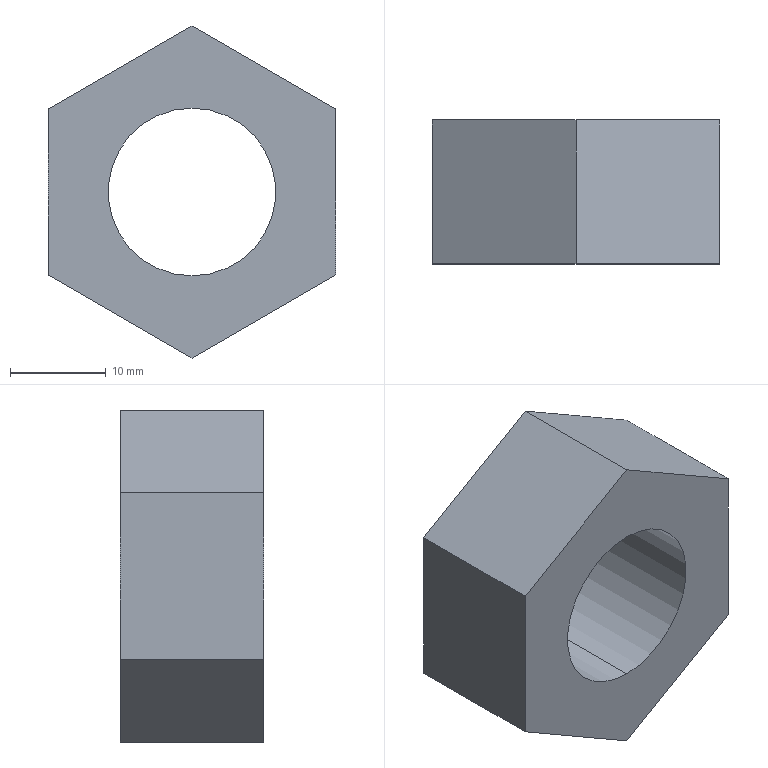Part | SolidWorks | features Extrusion 1, HoleWzd 1 | 1 solid | 10 faces | box 30 x 15 x 34.641 mm | volume 8083 mm3 | plane 8 | cylinder 2 | commonest cylinder face diameters 17.5 x2
STEP:
#1=CARTESIAN_POINT('',(0.,0.,-8.75));
#2=VERTEX_POINT('',#1);
#3=CARTESIAN_POINT('',(0.,0.,8.75));
#4=VERTEX_POINT('',#3);
#5=CARTESIAN_POINT('',(0.,0.,0.));
#6=DIRECTION('',(0.,1.,0.));
#7=DIRECTION('',(0.,0.,1.));
#8=AXIS2_PLACEMENT_3D('',#5,#6,#7);
#9=CIRCLE('',#8,8.75);
#10=EDGE_CURVE('',#2,#4,#9,.T.);
#11=ORIENTED_EDGE('',*,*,#10,.F.);
#12=CARTESIAN_POINT('',(0.,15.,-8.75));
#13=VERTEX_POINT('',#12);
#14=CARTESIAN_POINT('',(0.,15.,-8.75));
#15=DIRECTION('',(0.,1.,0.));
#16=VECTOR('',#15,1000.);
#17=LINE('',#14,#16);
#18=EDGE_CURVE('',#2,#13,#17,.T.);
#19=ORIENTED_EDGE('',*,*,#18,.T.);
#20=CARTESIAN_POINT('',(0.,15.,8.75));
#21=VERTEX_POINT('',#20);
#22=CARTESIAN_POINT('',(0.,15.,0.));
#23=DIRECTION('',(0.,1.,0.));
#24=DIRECTION('',(0.,0.,1.));
#25=AXIS2_PLACEMENT_3D('',#22,#23,#24);
#26=CIRCLE('',#25,8.75);
#27=EDGE_CURVE('',#13,#21,#26,.T.);
#28=ORIENTED_EDGE('',*,*,#27,.T.);
#29=CARTESIAN_POINT('',(0.,15.,8.75));
#30=DIRECTION('',(0.,1.,0.));
#31=VECTOR('',#30,1000.);
#32=LINE('',#29,#31);
#33=EDGE_CURVE('',#4,#21,#32,.T.);
#34=ORIENTED_EDGE('',*,*,#33,.F.);
#35=EDGE_LOOP('',(#11,#19,#28,#34));
#36=FACE_OUTER_BOUND('',#35,.T.);
#37=CARTESIAN_POINT('',(0.,15.,0.));
#38=DIRECTION('',(0.,1.,0.));
#39=DIRECTION('',(0.,0.,1.));
#40=AXIS2_PLACEMENT_3D('',#37,#38,#39);
#41=CYLINDRICAL_SURFACE('',#40,8.75);
#42=ADVANCED_FACE('',(#36),#41,.F.);
#43=CARTESIAN_POINT('',(15.,0.,-8.66));
#44=VERTEX_POINT('',#43);
#45=CARTESIAN_POINT('',(0.,0.,-17.321));
#46=VERTEX_POINT('',#45);
#47=CARTESIAN_POINT('',(15.,0.,-8.66));
#48=DIRECTION('',(-0.866,0.,-0.5));
#49=VECTOR('',#48,1000.);
#50=LINE('',#47,#49);
#51=EDGE_CURVE('',#44,#46,#50,.T.);
#52=ORIENTED_EDGE('',*,*,#51,.T.);
#53=CARTESIAN_POINT('',(0.,15.,-17.321));
#54=VERTEX_POINT('',#53);
#55=CARTESIAN_POINT('',(0.,15.,-17.321));
#56=DIRECTION('',(0.,-1.,0.));
#57=VECTOR('',#56,1000.);
#58=LINE('',#55,#57);
#59=EDGE_CURVE('',#54,#46,#58,.T.);
#60=ORIENTED_EDGE('',*,*,#59,.F.);
#61=CARTESIAN_POINT('',(15.,15.,-8.66));
#62=VERTEX_POINT('',#61);
#63=CARTESIAN_POINT('',(15.,15.,-8.66));
#64=DIRECTION('',(-0.866,0.,-0.5));
#65=VECTOR('',#64,1000.);
#66=LINE('',#63,#65);
#67=EDGE_CURVE('',#62,#54,#66,.T.);
#68=ORIENTED_EDGE('',*,*,#67,.F.);
#69=CARTESIAN_POINT('',(15.,15.,-8.66));
#70=DIRECTION('',(0.,-1.,0.));
#71=VECTOR('',#70,1000.);
#72=LINE('',#69,#71);
#73=EDGE_CURVE('',#62,#44,#72,.T.);
#74=ORIENTED_EDGE('',*,*,#73,.T.);
#75=EDGE_LOOP('',(#52,#60,#68,#74));
#76=FACE_OUTER_BOUND('',#75,.T.);
#77=CARTESIAN_POINT('',(15.,15.,-8.66));
#78=DIRECTION('',(-0.5,0.,0.866));
#79=DIRECTION('',(0.866,0.,0.5));
#80=AXIS2_PLACEMENT_3D('',#77,#78,#79);
#81=PLANE('',#80);
#82=ADVANCED_FACE('',(#76),#81,.F.);
#83=CARTESIAN_POINT('',(-15.,0.,-8.66));
#84=VERTEX_POINT('',#83);
#85=CARTESIAN_POINT('',(0.,0.,-17.321));
#86=DIRECTION('',(-0.866,0.,0.5));
#87=VECTOR('',#86,1000.);
#88=LINE('',#85,#87);
#89=EDGE_CURVE('',#46,#84,#88,.T.);
#90=ORIENTED_EDGE('',*,*,#89,.T.);
#91=CARTESIAN_POINT('',(-15.,15.,-8.66));
#92=VERTEX_POINT('',#91);
#93=CARTESIAN_POINT('',(-15.,15.,-8.66));
#94=DIRECTION('',(0.,-1.,0.));
#95=VECTOR('',#94,1000.);
#96=LINE('',#93,#95);
#97=EDGE_CURVE('',#92,#84,#96,.T.);
#98=ORIENTED_EDGE('',*,*,#97,.F.);
#99=CARTESIAN_POINT('',(0.,15.,-17.321));
#100=DIRECTION('',(-0.866,0.,0.5));
#101=VECTOR('',#100,1000.);
#102=LINE('',#99,#101);
#103=EDGE_CURVE('',#54,#92,#102,.T.);
#104=ORIENTED_EDGE('',*,*,#103,.F.);
#105=ORIENTED_EDGE('',*,*,#59,.T.);
#106=EDGE_LOOP('',(#90,#98,#104,#105));
#107=FACE_OUTER_BOUND('',#106,.T.);
#108=CARTESIAN_POINT('',(0.,15.,-17.321));
#109=DIRECTION('',(0.5,0.,0.866));
#110=DIRECTION('',(0.866,0.,-0.5));
#111=AXIS2_PLACEMENT_3D('',#108,#109,#110);
#112=PLANE('',#111);
#113=ADVANCED_FACE('',(#107),#112,.F.);
#114=CARTESIAN_POINT('',(-15.,0.,8.66));
#115=VERTEX_POINT('',#114);
#116=CARTESIAN_POINT('',(-15.,0.,-8.66));
#117=DIRECTION('',(0.,0.,1.));
#118=VECTOR('',#117,1000.);
#119=LINE('',#116,#118);
#120=EDGE_CURVE('',#84,#115,#119,.T.);
#121=ORIENTED_EDGE('',*,*,#120,.T.);
#122=CARTESIAN_POINT('',(-15.,15.,8.66));
#123=VERTEX_POINT('',#122);
#124=CARTESIAN_POINT('',(-15.,15.,8.66));
#125=DIRECTION('',(0.,-1.,0.));
#126=VECTOR('',#125,1000.);
#127=LINE('',#124,#126);
#128=EDGE_CURVE('',#123,#115,#127,.T.);
#129=ORIENTED_EDGE('',*,*,#128,.F.);
#130=CARTESIAN_POINT('',(-15.,15.,-8.66));
#131=DIRECTION('',(0.,0.,1.));
#132=VECTOR('',#131,1000.);
#133=LINE('',#130,#132);
#134=EDGE_CURVE('',#92,#123,#133,.T.);
#135=ORIENTED_EDGE('',*,*,#134,.F.);
#136=ORIENTED_EDGE('',*,*,#97,.T.);
#137=EDGE_LOOP('',(#121,#129,#135,#136));
#138=FACE_OUTER_BOUND('',#137,.T.);
#139=CARTESIAN_POINT('',(-15.,15.,-8.66));
#140=DIRECTION('',(1.,0.,0.));
#141=DIRECTION('',(0.,0.,-1.));
#142=AXIS2_PLACEMENT_3D('',#139,#140,#141);
#143=PLANE('',#142);
#144=ADVANCED_FACE('',(#138),#143,.F.);
#145=CARTESIAN_POINT('',(0.,0.,17.321));
#146=VERTEX_POINT('',#145);
#147=CARTESIAN_POINT('',(-15.,0.,8.66));
#148=DIRECTION('',(0.866,0.,0.5));
#149=VECTOR('',#148,1000.);
#150=LINE('',#147,#149);
#151=EDGE_CURVE('',#115,#146,#150,.T.);
#152=ORIENTED_EDGE('',*,*,#151,.T.);
#153=CARTESIAN_POINT('',(0.,15.,17.321));
#154=VERTEX_POINT('',#153);
#155=CARTESIAN_POINT('',(0.,15.,17.321));
#156=DIRECTION('',(0.,-1.,0.));
#157=VECTOR('',#156,1000.);
#158=LINE('',#155,#157);
#159=EDGE_CURVE('',#154,#146,#158,.T.);
#160=ORIENTED_EDGE('',*,*,#159,.F.);
#161=CARTESIAN_POINT('',(-15.,15.,8.66));
#162=DIRECTION('',(0.866,0.,0.5));
#163=VECTOR('',#162,1000.);
#164=LINE('',#161,#163);
#165=EDGE_CURVE('',#123,#154,#164,.T.);
#166=ORIENTED_EDGE('',*,*,#165,.F.);
#167=ORIENTED_EDGE('',*,*,#128,.T.);
#168=EDGE_LOOP('',(#152,#160,#166,#167));
#169=FACE_OUTER_BOUND('',#168,.T.);
#170=CARTESIAN_POINT('',(-15.,15.,8.66));
#171=DIRECTION('',(0.5,0.,-0.866));
#172=DIRECTION('',(-0.866,0.,-0.5));
#173=AXIS2_PLACEMENT_3D('',#170,#171,#172);
#174=PLANE('',#173);
#175=ADVANCED_FACE('',(#169),#174,.F.);
#176=CARTESIAN_POINT('',(15.,0.,8.66));
#177=VERTEX_POINT('',#176);
#178=CARTESIAN_POINT('',(0.,0.,17.321));
#179=DIRECTION('',(0.866,0.,-0.5));
#180=VECTOR('',#179,1000.);
#181=LINE('',#178,#180);
#182=EDGE_CURVE('',#146,#177,#181,.T.);
#183=ORIENTED_EDGE('',*,*,#182,.T.);
#184=CARTESIAN_POINT('',(15.,15.,8.66));
#185=VERTEX_POINT('',#184);
#186=CARTESIAN_POINT('',(15.,15.,8.66));
#187=DIRECTION('',(0.,-1.,0.));
#188=VECTOR('',#187,1000.);
#189=LINE('',#186,#188);
#190=EDGE_CURVE('',#185,#177,#189,.T.);
#191=ORIENTED_EDGE('',*,*,#190,.F.);
#192=CARTESIAN_POINT('',(0.,15.,17.321));
#193=DIRECTION('',(0.866,0.,-0.5));
#194=VECTOR('',#193,1000.);
#195=LINE('',#192,#194);
#196=EDGE_CURVE('',#154,#185,#195,.T.);
#197=ORIENTED_EDGE('',*,*,#196,.F.);
#198=ORIENTED_EDGE('',*,*,#159,.T.);
#199=EDGE_LOOP('',(#183,#191,#197,#198));
#200=FACE_OUTER_BOUND('',#199,.T.);
#201=CARTESIAN_POINT('',(0.,15.,17.321));
#202=DIRECTION('',(-0.5,0.,-0.866));
#203=DIRECTION('',(-0.866,0.,0.5));
#204=AXIS2_PLACEMENT_3D('',#201,#202,#203);
#205=PLANE('',#204);
#206=ADVANCED_FACE('',(#200),#205,.F.);
#207=CARTESIAN_POINT('',(15.,0.,8.66));
#208=DIRECTION('',(0.,0.,-1.));
#209=VECTOR('',#208,1000.);
#210=LINE('',#207,#209);
#211=EDGE_CURVE('',#177,#44,#210,.T.);
#212=ORIENTED_EDGE('',*,*,#211,.T.);
#213=ORIENTED_EDGE('',*,*,#73,.F.);
#214=CARTESIAN_POINT('',(15.,15.,8.66));
#215=DIRECTION('',(0.,0.,-1.));
#216=VECTOR('',#215,1000.);
#217=LINE('',#214,#216);
#218=EDGE_CURVE('',#185,#62,#217,.T.);
#219=ORIENTED_EDGE('',*,*,#218,.F.);
#220=ORIENTED_EDGE('',*,*,#190,.T.);
#221=EDGE_LOOP('',(#212,#213,#219,#220));
#222=FACE_OUTER_BOUND('',#221,.T.);
#223=CARTESIAN_POINT('',(15.,15.,8.66));
#224=DIRECTION('',(-1.,0.,0.));
#225=DIRECTION('',(0.,0.,1.));
#226=AXIS2_PLACEMENT_3D('',#223,#224,#225);
#227=PLANE('',#226);
#228=ADVANCED_FACE('',(#222),#227,.F.);
#229=CARTESIAN_POINT('',(0.,15.,0.));
#230=DIRECTION('',(0.,1.,0.));
#231=DIRECTION('',(0.,0.,1.));
#232=AXIS2_PLACEMENT_3D('',#229,#230,#231);
#233=CIRCLE('',#232,8.75);
#234=EDGE_CURVE('',#21,#13,#233,.T.);
#235=ORIENTED_EDGE('',*,*,#234,.F.);
#236=ORIENTED_EDGE('',*,*,#27,.F.);
#237=EDGE_LOOP('',(#235,#236));
#238=FACE_BOUND('',#237,.T.);
#239=ORIENTED_EDGE('',*,*,#67,.T.);
#240=ORIENTED_EDGE('',*,*,#103,.T.);
#241=ORIENTED_EDGE('',*,*,#134,.T.);
#242=ORIENTED_EDGE('',*,*,#165,.T.);
#243=ORIENTED_EDGE('',*,*,#196,.T.);
#244=ORIENTED_EDGE('',*,*,#218,.T.);
#245=EDGE_LOOP('',(#239,#240,#241,#242,#243,#244));
#246=FACE_OUTER_BOUND('',#245,.T.);
#247=CARTESIAN_POINT('',(0.,15.,0.));
#248=DIRECTION('',(0.,1.,0.));
#249=DIRECTION('',(0.,0.,1.));
#250=AXIS2_PLACEMENT_3D('',#247,#248,#249);
#251=PLANE('',#250);
#252=ADVANCED_FACE('',(#238,#246),#251,.T.);
#253=CARTESIAN_POINT('',(0.,0.,0.));
#254=DIRECTION('',(0.,1.,0.));
#255=DIRECTION('',(0.,0.,1.));
#256=AXIS2_PLACEMENT_3D('',#253,#254,#255);
#257=CIRCLE('',#256,8.75);
#258=EDGE_CURVE('',#4,#2,#257,.T.);
#259=ORIENTED_EDGE('',*,*,#258,.T.);
#260=ORIENTED_EDGE('',*,*,#10,.T.);
#261=EDGE_LOOP('',(#259,#260));
#262=FACE_BOUND('',#261,.T.);
#263=ORIENTED_EDGE('',*,*,#51,.F.);
#264=ORIENTED_EDGE('',*,*,#211,.F.);
#265=ORIENTED_EDGE('',*,*,#182,.F.);
#266=ORIENTED_EDGE('',*,*,#151,.F.);
#267=ORIENTED_EDGE('',*,*,#120,.F.);
#268=ORIENTED_EDGE('',*,*,#89,.F.);
#269=EDGE_LOOP('',(#263,#264,#265,#266,#267,#268));
#270=FACE_OUTER_BOUND('',#269,.T.);
#271=CARTESIAN_POINT('',(0.,0.,0.));
#272=DIRECTION('',(0.,1.,0.));
#273=DIRECTION('',(0.,0.,1.));
#274=AXIS2_PLACEMENT_3D('',#271,#272,#273);
#275=PLANE('',#274);
#276=ADVANCED_FACE('',(#262,#270),#275,.F.);
#277=ORIENTED_EDGE('',*,*,#18,.F.);
#278=ORIENTED_EDGE('',*,*,#258,.F.);
#279=ORIENTED_EDGE('',*,*,#33,.T.);
#280=ORIENTED_EDGE('',*,*,#234,.T.);
#281=EDGE_LOOP('',(#277,#278,#279,#280));
#282=FACE_OUTER_BOUND('',#281,.T.);
#283=CARTESIAN_POINT('',(0.,15.,0.));
#284=DIRECTION('',(0.,1.,0.));
#285=DIRECTION('',(0.,0.,1.));
#286=AXIS2_PLACEMENT_3D('',#283,#284,#285);
#287=CYLINDRICAL_SURFACE('',#286,8.75);
#288=ADVANCED_FACE('',(#282),#287,.F.);
#289=CLOSED_SHELL('',(#42,#82,#113,#144,#175,#206,#228,#252,#276,#288));
#290=MANIFOLD_SOLID_BREP('',#289);
#291=CARTESIAN_POINT('',(0.,0.,0.));
#292=DIRECTION('',(0.,0.,1.));
#293=DIRECTION('',(1.,0.,0.));
#294=AXIS2_PLACEMENT_3D('',#291,#292,#293);
#295=(LENGTH_UNIT()NAMED_UNIT(*)SI_UNIT(.MILLI.,.METRE.));
#296=UNCERTAINTY_MEASURE_WITH_UNIT(LENGTH_MEASURE(0.00001),#295,'','');
#297=(NAMED_UNIT(*)PLANE_ANGLE_UNIT()SI_UNIT($,.RADIAN.));
#298=(NAMED_UNIT(*)SI_UNIT($,.STERADIAN.)SOLID_ANGLE_UNIT());
#299=(GEOMETRIC_REPRESENTATION_CONTEXT(3)GLOBAL_UNCERTAINTY_ASSIGNED_CONTEXT((#296))GLOBAL_UNIT_ASSIGNED_CONTEXT((#295,#297,#298))REPRESENTATION_CONTEXT('',''));
#300=ADVANCED_BREP_SHAPE_REPRESENTATION('',(#290,#294),#299);